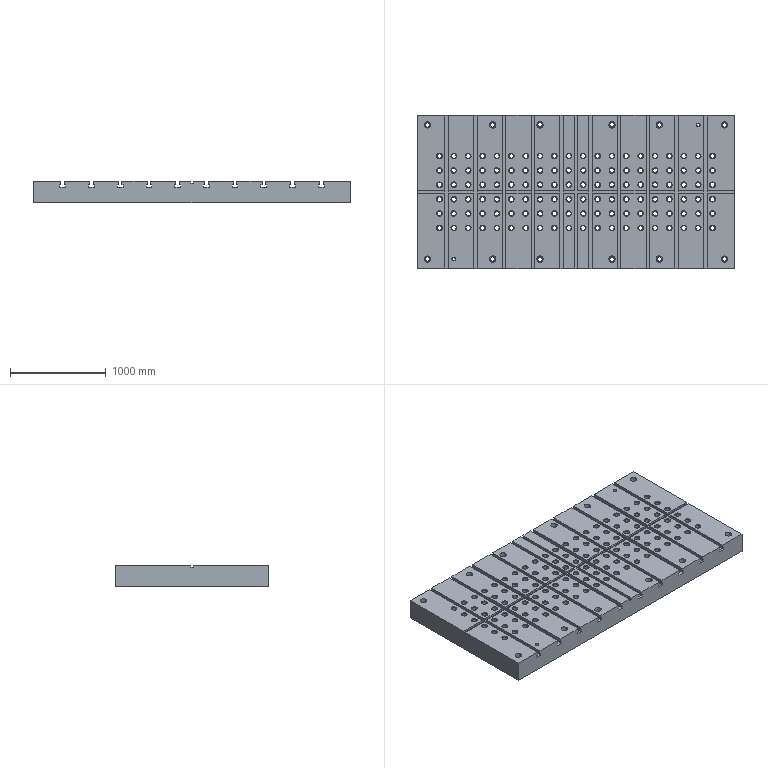Part | NX | features solid 2 | 1 solid | 540 faces | box 3300 x 1600 x 220 mm | volume 1059682394 mm3 | plane 272 | cylinder 268 | commonest cylinder face diameters 48 x120 60 x120 45 x12 68 x12 30 x2 40 x2